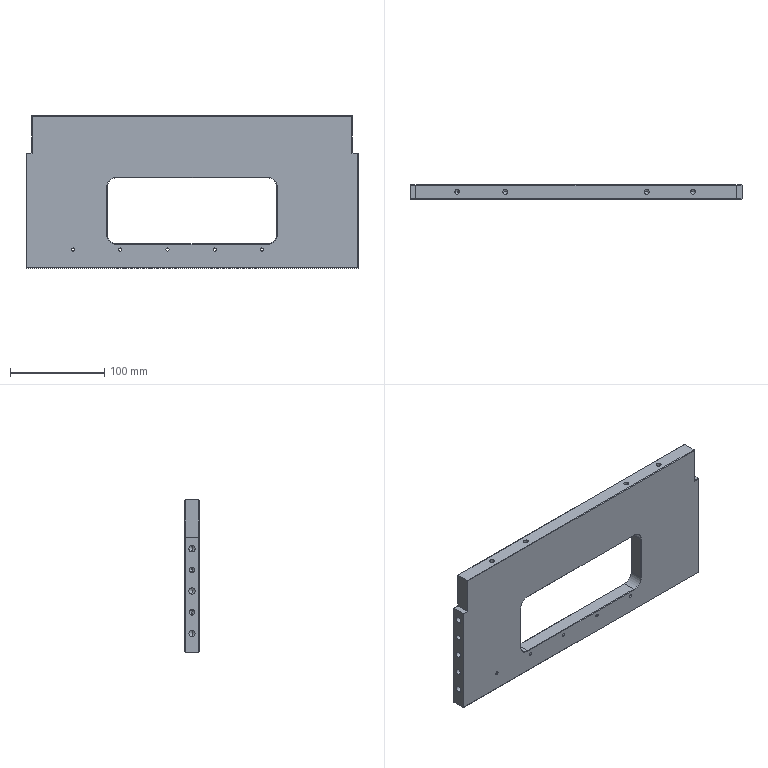Part | STEP file | 11-FG-SJ00411 | 1 solid | 116 faces | box 352 x 15 x 162 mm | volume 652972 mm3 | cylinder 42 | plane 38 | cone 36 | commonest cylinder face diameters 6.8 x12 3.3 x10 5 x8 6 x8 20 x4